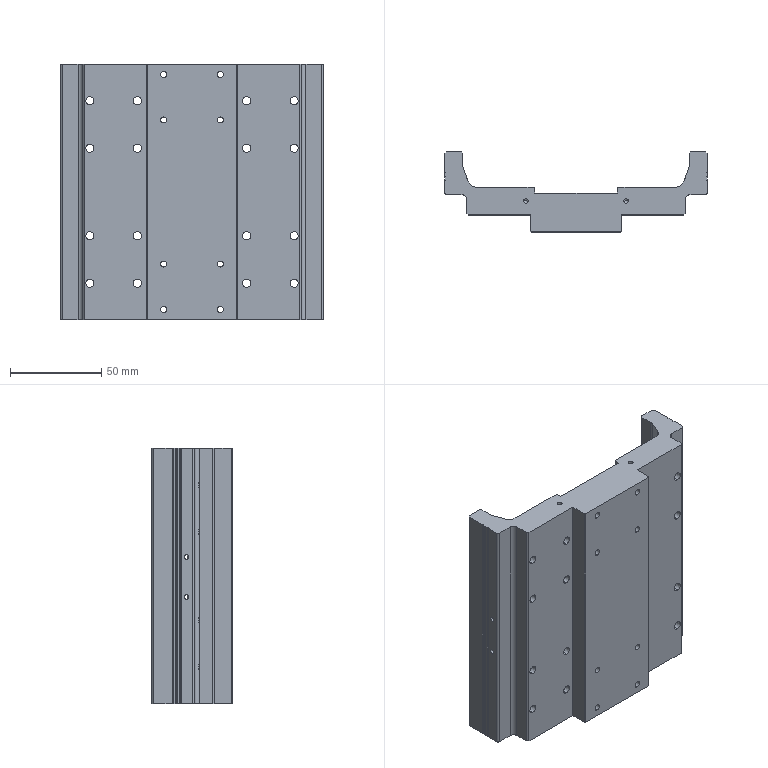Part | SolidWorks | features BaseBody 1 | 1 solid | 248 faces | box 144 x 44 x 140 mm | volume 348731 mm3 | cylinder 140 | plane 72 | cone 36 | commonest cylinder face diameters 4.5 x32 8 x32 2.5 x20 3.3 x16 6 x12 6.8 x12